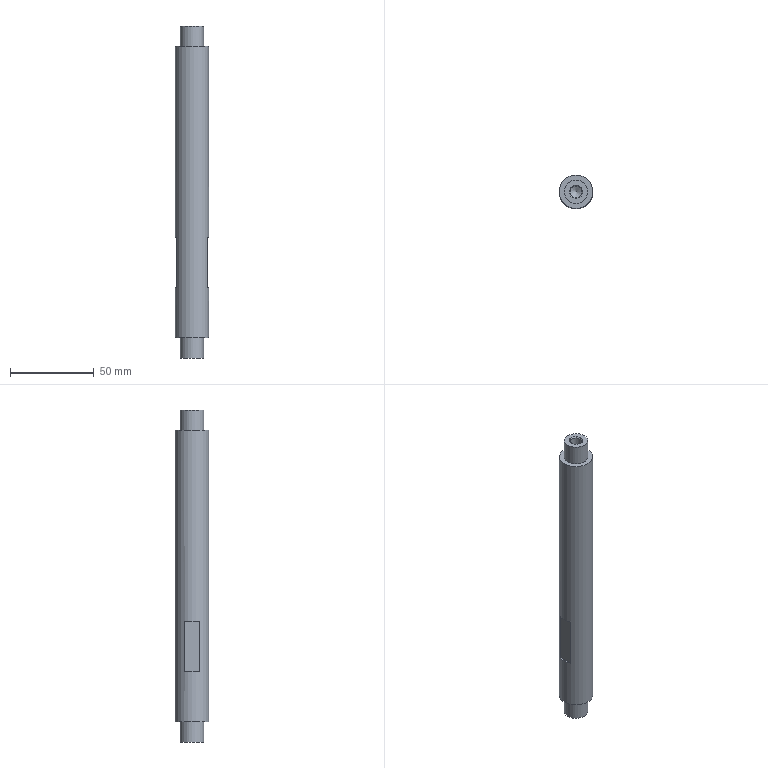Part | STEP file | YBQDJ-YL-9 | 1 solid | 16 faces | box 20 x 20 x 198 mm | volume 57396 mm3 | plane 10 | cylinder 4 | cone 2 | commonest cylinder face diameters 14 x2 6.8 x1 20 x1
STEP:
#1=CARTESIAN_POINT('',(0.,0.,0.));
#2=DIRECTION('',(0.,0.,1.));
#3=DIRECTION('',(1.,0.,0.));
#4=AXIS2_PLACEMENT_3D('',#1,#2,#3);
#5=CARTESIAN_POINT('',(231.5,-285.,50.));
#6=VERTEX_POINT('',#5);
#7=CARTESIAN_POINT('',(230.5,-280.641,50.));
#8=VERTEX_POINT('',#7);
#9=CARTESIAN_POINT('',(221.5,-285.,50.));
#10=DIRECTION('',(0.,0.,1.));
#11=DIRECTION('',(1.,0.,0.));
#12=AXIS2_PLACEMENT_3D('',#9,#10,#11);
#13=CIRCLE('',#12,10.);
#14=CARTESIAN_POINT('',(221.5,-285.,311.));
#15=DIRECTION('',(0.,0.,-1.));
#16=DIRECTION('',(1.,0.,0.));
#17=AXIS2_PLACEMENT_3D('',#14,#15,#16);
#18=CYLINDRICAL_SURFACE('',#17,10.);
#19=CARTESIAN_POINT('',(12.566,261.));
#20=DIRECTION('',(-1.,0.));
#21=VECTOR('',#20,1.);
#22=LINE('',#19,#21);
#23=(GEOMETRIC_REPRESENTATION_CONTEXT(2)PARAMETRIC_REPRESENTATION_CONTEXT()REPRESENTATION_CONTEXT('',''));
#24=DEFINITIONAL_REPRESENTATION('',(#22),#23);
#25=PCURVE('',#18,#24);
#26=CARTESIAN_POINT('',(230.5,-350.,50.));
#27=DIRECTION('',(0.,0.,1.));
#28=DIRECTION('',(1.,0.,0.));
#29=AXIS2_PLACEMENT_3D('',#26,#27,#28);
#30=PLANE('',#29);
#31=CARTESIAN_POINT('',(-9.,65.));
#32=DIRECTION('',(1.,0.));
#33=AXIS2_PLACEMENT_2D('',#31,#32);
#34=CIRCLE('',#33,10.);
#35=(GEOMETRIC_REPRESENTATION_CONTEXT(2)PARAMETRIC_REPRESENTATION_CONTEXT()REPRESENTATION_CONTEXT('',''));
#36=DEFINITIONAL_REPRESENTATION('',(#34),#35);
#37=PCURVE('',#30,#36);
#38=SURFACE_CURVE('',#13,(#25,#37),.PCURVE_S1.);
#39=EDGE_CURVE('',#6,#8,#38,.T.);
#40=ORIENTED_EDGE('',*,*,#39,.F.);
#41=CARTESIAN_POINT('',(231.5,-285.,20.));
#42=VERTEX_POINT('',#41);
#43=CARTESIAN_POINT('',(231.5,-285.,50.));
#44=CARTESIAN_POINT('',(231.5,-285.,20.));
#45=B_SPLINE_CURVE_WITH_KNOTS('',1,(#43,#44),.UNSPECIFIED.,.F.,.F.,(2,2),(261.,291.),.PIECEWISE_BEZIER_KNOTS.);
#46=CARTESIAN_POINT('',(6.283,0.));
#47=DIRECTION('',(0.,1.));
#48=VECTOR('',#47,1.);
#49=LINE('',#46,#48);
#50=(GEOMETRIC_REPRESENTATION_CONTEXT(2)PARAMETRIC_REPRESENTATION_CONTEXT()REPRESENTATION_CONTEXT('',''));
#51=DEFINITIONAL_REPRESENTATION('',(#49),#50);
#52=PCURVE('',#18,#51);
#53=CARTESIAN_POINT('',(0.,0.));
#54=DIRECTION('',(0.,1.));
#55=VECTOR('',#54,1.);
#56=LINE('',#53,#55);
#57=(GEOMETRIC_REPRESENTATION_CONTEXT(2)PARAMETRIC_REPRESENTATION_CONTEXT()REPRESENTATION_CONTEXT('',''));
#58=DEFINITIONAL_REPRESENTATION('',(#56),#57);
#59=PCURVE('',#18,#58);
#60=SEAM_CURVE('',#45,(#52,#59),.PCURVE_S1.);
#61=EDGE_CURVE('',#6,#42,#60,.T.);
#62=ORIENTED_EDGE('',*,*,#61,.T.);
#63=CARTESIAN_POINT('',(221.5,-285.,20.));
#64=DIRECTION('',(0.,0.,1.));
#65=DIRECTION('',(1.,0.,0.));
#66=AXIS2_PLACEMENT_3D('',#63,#64,#65);
#67=CIRCLE('',#66,10.);
#68=CARTESIAN_POINT('',(6.283,291.));
#69=DIRECTION('',(-1.,0.));
#70=VECTOR('',#69,1.);
#71=LINE('',#68,#70);
#72=(GEOMETRIC_REPRESENTATION_CONTEXT(2)PARAMETRIC_REPRESENTATION_CONTEXT()REPRESENTATION_CONTEXT('',''));
#73=DEFINITIONAL_REPRESENTATION('',(#71),#72);
#74=PCURVE('',#18,#73);
#75=CARTESIAN_POINT('',(131.5,-90.,20.));
#76=DIRECTION('',(0.,0.,1.));
#77=DIRECTION('',(0.,-1.,0.));
#78=AXIS2_PLACEMENT_3D('',#75,#76,#77);
#79=PLANE('',#78);
#80=CARTESIAN_POINT('',(195.,90.));
#81=DIRECTION('',(0.,1.));
#82=AXIS2_PLACEMENT_2D('',#80,#81);
#83=CIRCLE('',#82,10.);
#84=(GEOMETRIC_REPRESENTATION_CONTEXT(2)PARAMETRIC_REPRESENTATION_CONTEXT()REPRESENTATION_CONTEXT('',''));
#85=DEFINITIONAL_REPRESENTATION('',(#83),#84);
#86=PCURVE('',#79,#85);
#87=SURFACE_CURVE('',#67,(#74,#86),.PCURVE_S1.);
#88=EDGE_CURVE('',#42,#42,#87,.T.);
#89=ORIENTED_EDGE('',*,*,#88,.T.);
#90=ORIENTED_EDGE('',*,*,#61,.F.);
#91=CARTESIAN_POINT('',(230.5,-289.359,50.));
#92=VERTEX_POINT('',#91);
#93=CARTESIAN_POINT('',(221.5,-285.,50.));
#94=DIRECTION('',(0.,0.,1.));
#95=DIRECTION('',(1.,0.,0.));
#96=AXIS2_PLACEMENT_3D('',#93,#94,#95);
#97=CIRCLE('',#96,10.);
#98=CARTESIAN_POINT('',(6.283,261.));
#99=DIRECTION('',(-1.,0.));
#100=VECTOR('',#99,1.);
#101=LINE('',#98,#100);
#102=(GEOMETRIC_REPRESENTATION_CONTEXT(2)PARAMETRIC_REPRESENTATION_CONTEXT()REPRESENTATION_CONTEXT('',''));
#103=DEFINITIONAL_REPRESENTATION('',(#101),#102);
#104=PCURVE('',#18,#103);
#105=CARTESIAN_POINT('',(-9.,65.));
#106=DIRECTION('',(1.,0.));
#107=AXIS2_PLACEMENT_2D('',#105,#106);
#108=CIRCLE('',#107,10.);
#109=(GEOMETRIC_REPRESENTATION_CONTEXT(2)PARAMETRIC_REPRESENTATION_CONTEXT()REPRESENTATION_CONTEXT('',''));
#110=DEFINITIONAL_REPRESENTATION('',(#108),#109);
#111=PCURVE('',#30,#110);
#112=SURFACE_CURVE('',#97,(#104,#111),.PCURVE_S1.);
#113=EDGE_CURVE('',#92,#6,#112,.T.);
#114=ORIENTED_EDGE('',*,*,#113,.F.);
#115=CARTESIAN_POINT('',(230.5,-289.359,80.));
#116=VERTEX_POINT('',#115);
#117=CARTESIAN_POINT('',(230.5,-289.359,311.));
#118=DIRECTION('',(0.,0.,-1.));
#119=VECTOR('',#118,1.);
#120=LINE('',#117,#119);
#121=CARTESIAN_POINT('',(0.451,0.));
#122=DIRECTION('',(0.,1.));
#123=VECTOR('',#122,1.);
#124=LINE('',#121,#123);
#125=(GEOMETRIC_REPRESENTATION_CONTEXT(2)PARAMETRIC_REPRESENTATION_CONTEXT()REPRESENTATION_CONTEXT('',''));
#126=DEFINITIONAL_REPRESENTATION('',(#124),#125);
#127=PCURVE('',#18,#126);
#128=CARTESIAN_POINT('',(230.5,-350.,80.));
#129=DIRECTION('',(1.,0.,0.));
#130=DIRECTION('',(0.,0.,-1.));
#131=AXIS2_PLACEMENT_3D('',#128,#129,#130);
#132=PLANE('',#131);
#133=CARTESIAN_POINT('',(-231.,60.641));
#134=DIRECTION('',(1.,0.));
#135=VECTOR('',#134,1.);
#136=LINE('',#133,#135);
#137=(GEOMETRIC_REPRESENTATION_CONTEXT(2)PARAMETRIC_REPRESENTATION_CONTEXT()REPRESENTATION_CONTEXT('',''));
#138=DEFINITIONAL_REPRESENTATION('',(#136),#137);
#139=PCURVE('',#132,#138);
#140=SURFACE_CURVE('',#120,(#127,#139),.PCURVE_S1.);
#141=EDGE_CURVE('',#116,#92,#140,.T.);
#142=ORIENTED_EDGE('',*,*,#141,.F.);
#143=CARTESIAN_POINT('',(231.5,-285.,80.));
#144=VERTEX_POINT('',#143);
#145=CARTESIAN_POINT('',(221.5,-285.,80.));
#146=DIRECTION('',(0.,0.,-1.));
#147=DIRECTION('',(-1.,0.,0.));
#148=AXIS2_PLACEMENT_3D('',#145,#146,#147);
#149=CIRCLE('',#148,10.);
#150=CARTESIAN_POINT('',(-3.142,231.));
#151=DIRECTION('',(1.,0.));
#152=VECTOR('',#151,1.);
#153=LINE('',#150,#152);
#154=(GEOMETRIC_REPRESENTATION_CONTEXT(2)PARAMETRIC_REPRESENTATION_CONTEXT()REPRESENTATION_CONTEXT('',''));
#155=DEFINITIONAL_REPRESENTATION('',(#153),#154);
#156=PCURVE('',#18,#155);
#157=CARTESIAN_POINT('',(259.,-350.,80.));
#158=DIRECTION('',(0.,0.,-1.));
#159=DIRECTION('',(-1.,0.,0.));
#160=AXIS2_PLACEMENT_3D('',#157,#158,#159);
#161=PLANE('',#160);
#162=CARTESIAN_POINT('',(37.5,65.));
#163=DIRECTION('',(1.,0.));
#164=AXIS2_PLACEMENT_2D('',#162,#163);
#165=CIRCLE('',#164,10.);
#166=(GEOMETRIC_REPRESENTATION_CONTEXT(2)PARAMETRIC_REPRESENTATION_CONTEXT()REPRESENTATION_CONTEXT('',''));
#167=DEFINITIONAL_REPRESENTATION('',(#165),#166);
#168=PCURVE('',#161,#167);
#169=SURFACE_CURVE('',#149,(#156,#168),.PCURVE_S1.);
#170=EDGE_CURVE('',#144,#116,#169,.T.);
#171=ORIENTED_EDGE('',*,*,#170,.F.);
#172=CARTESIAN_POINT('',(231.5,-285.,194.));
#173=VERTEX_POINT('',#172);
#174=CARTESIAN_POINT('',(231.5,-285.,194.));
#175=CARTESIAN_POINT('',(231.5,-285.,80.));
#176=B_SPLINE_CURVE_WITH_KNOTS('',1,(#174,#175),.UNSPECIFIED.,.F.,.F.,(2,2),(117.,231.),.PIECEWISE_BEZIER_KNOTS.);
#177=CARTESIAN_POINT('',(0.,0.));
#178=DIRECTION('',(0.,1.));
#179=VECTOR('',#178,1.);
#180=LINE('',#177,#179);
#181=(GEOMETRIC_REPRESENTATION_CONTEXT(2)PARAMETRIC_REPRESENTATION_CONTEXT()REPRESENTATION_CONTEXT('',''));
#182=DEFINITIONAL_REPRESENTATION('',(#180),#181);
#183=PCURVE('',#18,#182);
#184=CARTESIAN_POINT('',(6.283,0.));
#185=DIRECTION('',(0.,1.));
#186=VECTOR('',#185,1.);
#187=LINE('',#184,#186);
#188=(GEOMETRIC_REPRESENTATION_CONTEXT(2)PARAMETRIC_REPRESENTATION_CONTEXT()REPRESENTATION_CONTEXT('',''));
#189=DEFINITIONAL_REPRESENTATION('',(#187),#188);
#190=PCURVE('',#18,#189);
#191=SEAM_CURVE('',#176,(#183,#190),.PCURVE_S1.);
#192=EDGE_CURVE('',#173,#144,#191,.T.);
#193=ORIENTED_EDGE('',*,*,#192,.F.);
#194=CARTESIAN_POINT('',(211.5,-285.,194.));
#195=VERTEX_POINT('',#194);
#196=CARTESIAN_POINT('',(221.5,-285.,194.));
#197=DIRECTION('',(0.,0.,1.));
#198=DIRECTION('',(-1.,0.,0.));
#199=AXIS2_PLACEMENT_3D('',#196,#197,#198);
#200=CIRCLE('',#199,10.);
#201=CARTESIAN_POINT('',(3.142,117.));
#202=DIRECTION('',(-1.,0.));
#203=VECTOR('',#202,1.);
#204=LINE('',#201,#203);
#205=(GEOMETRIC_REPRESENTATION_CONTEXT(2)PARAMETRIC_REPRESENTATION_CONTEXT()REPRESENTATION_CONTEXT('',''));
#206=DEFINITIONAL_REPRESENTATION('',(#204),#205);
#207=PCURVE('',#18,#206);
#208=CARTESIAN_POINT('',(365.5,-285.,194.));
#209=DIRECTION('',(0.,0.,-1.));
#210=DIRECTION('',(-1.,0.,0.));
#211=AXIS2_PLACEMENT_3D('',#208,#209,#210);
#212=PLANE('',#211);
#213=CARTESIAN_POINT('',(154.,0.));
#214=CARTESIAN_POINT('',(154.,-17.321));
#215=CARTESIAN_POINT('',(139.,-8.66));
#216=CARTESIAN_POINT('',(124.,0.));
#217=CARTESIAN_POINT('',(139.,8.66));
#218=CARTESIAN_POINT('',(154.,17.321));
#219=CARTESIAN_POINT('',(154.,0.));
#220=(BOUNDED_CURVE()B_SPLINE_CURVE(2,(#213,#214,#215,#216,#217,#218,#219),.UNSPECIFIED.,.T.,.F.)B_SPLINE_CURVE_WITH_KNOTS((1,2,2,2,2,1),(-2.094,0.,2.094,4.189,6.283,8.378),.UNSPECIFIED.)CURVE()GEOMETRIC_REPRESENTATION_ITEM()RATIONAL_B_SPLINE_CURVE((1.,0.5,1.,0.5,1.,0.5,1.))REPRESENTATION_ITEM(''));
#221=(GEOMETRIC_REPRESENTATION_CONTEXT(2)PARAMETRIC_REPRESENTATION_CONTEXT()REPRESENTATION_CONTEXT('',''));
#222=DEFINITIONAL_REPRESENTATION('',(#220),#221);
#223=PCURVE('',#212,#222);
#224=SURFACE_CURVE('',#200,(#207,#223),.PCURVE_S1.);
#225=EDGE_CURVE('',#195,#173,#224,.T.);
#226=ORIENTED_EDGE('',*,*,#225,.F.);
#227=CARTESIAN_POINT('',(221.5,-285.,194.));
#228=DIRECTION('',(0.,0.,1.));
#229=DIRECTION('',(-1.,0.,0.));
#230=AXIS2_PLACEMENT_3D('',#227,#228,#229);
#231=CIRCLE('',#230,10.);
#232=CARTESIAN_POINT('',(9.425,117.));
#233=DIRECTION('',(-1.,0.));
#234=VECTOR('',#233,1.);
#235=LINE('',#232,#234);
#236=(GEOMETRIC_REPRESENTATION_CONTEXT(2)PARAMETRIC_REPRESENTATION_CONTEXT()REPRESENTATION_CONTEXT('',''));
#237=DEFINITIONAL_REPRESENTATION('',(#235),#236);
#238=PCURVE('',#18,#237);
#239=CARTESIAN_POINT('',(154.,0.));
#240=CARTESIAN_POINT('',(154.,-17.321));
#241=CARTESIAN_POINT('',(139.,-8.66));
#242=CARTESIAN_POINT('',(124.,0.));
#243=CARTESIAN_POINT('',(139.,8.66));
#244=CARTESIAN_POINT('',(154.,17.321));
#245=CARTESIAN_POINT('',(154.,0.));
#246=(BOUNDED_CURVE()B_SPLINE_CURVE(2,(#239,#240,#241,#242,#243,#244,#245),.UNSPECIFIED.,.T.,.F.)B_SPLINE_CURVE_WITH_KNOTS((1,2,2,2,2,1),(-2.094,0.,2.094,4.189,6.283,8.378),.UNSPECIFIED.)CURVE()GEOMETRIC_REPRESENTATION_ITEM()RATIONAL_B_SPLINE_CURVE((1.,0.5,1.,0.5,1.,0.5,1.))REPRESENTATION_ITEM(''));
#247=(GEOMETRIC_REPRESENTATION_CONTEXT(2)PARAMETRIC_REPRESENTATION_CONTEXT()REPRESENTATION_CONTEXT('',''));
#248=DEFINITIONAL_REPRESENTATION('',(#246),#247);
#249=PCURVE('',#212,#248);
#250=SURFACE_CURVE('',#231,(#238,#249),.PCURVE_S1.);
#251=EDGE_CURVE('',#173,#195,#250,.T.);
#252=ORIENTED_EDGE('',*,*,#251,.F.);
#253=ORIENTED_EDGE('',*,*,#192,.T.);
#254=CARTESIAN_POINT('',(230.5,-280.641,80.));
#255=VERTEX_POINT('',#254);
#256=CARTESIAN_POINT('',(221.5,-285.,80.));
#257=DIRECTION('',(0.,0.,-1.));
#258=DIRECTION('',(-1.,0.,0.));
#259=AXIS2_PLACEMENT_3D('',#256,#257,#258);
#260=CIRCLE('',#259,10.);
#261=CARTESIAN_POINT('',(3.142,231.));
#262=DIRECTION('',(1.,0.));
#263=VECTOR('',#262,1.);
#264=LINE('',#261,#263);
#265=(GEOMETRIC_REPRESENTATION_CONTEXT(2)PARAMETRIC_REPRESENTATION_CONTEXT()REPRESENTATION_CONTEXT('',''));
#266=DEFINITIONAL_REPRESENTATION('',(#264),#265);
#267=PCURVE('',#18,#266);
#268=CARTESIAN_POINT('',(37.5,65.));
#269=DIRECTION('',(1.,0.));
#270=AXIS2_PLACEMENT_2D('',#268,#269);
#271=CIRCLE('',#270,10.);
#272=(GEOMETRIC_REPRESENTATION_CONTEXT(2)PARAMETRIC_REPRESENTATION_CONTEXT()REPRESENTATION_CONTEXT('',''));
#273=DEFINITIONAL_REPRESENTATION('',(#271),#272);
#274=PCURVE('',#161,#273);
#275=SURFACE_CURVE('',#260,(#267,#274),.PCURVE_S1.);
#276=EDGE_CURVE('',#255,#144,#275,.T.);
#277=ORIENTED_EDGE('',*,*,#276,.F.);
#278=CARTESIAN_POINT('',(230.5,-280.641,311.));
#279=DIRECTION('',(0.,0.,1.));
#280=VECTOR('',#279,1.);
#281=LINE('',#278,#280);
#282=CARTESIAN_POINT('',(5.832,0.));
#283=DIRECTION('',(0.,-1.));
#284=VECTOR('',#283,1.);
#285=LINE('',#282,#284);
#286=(GEOMETRIC_REPRESENTATION_CONTEXT(2)PARAMETRIC_REPRESENTATION_CONTEXT()REPRESENTATION_CONTEXT('',''));
#287=DEFINITIONAL_REPRESENTATION('',(#285),#286);
#288=PCURVE('',#18,#287);
#289=CARTESIAN_POINT('',(-231.,69.359));
#290=DIRECTION('',(-1.,0.));
#291=VECTOR('',#290,1.);
#292=LINE('',#289,#291);
#293=(GEOMETRIC_REPRESENTATION_CONTEXT(2)PARAMETRIC_REPRESENTATION_CONTEXT()REPRESENTATION_CONTEXT('',''));
#294=DEFINITIONAL_REPRESENTATION('',(#292),#293);
#295=PCURVE('',#132,#294);
#296=SURFACE_CURVE('',#281,(#288,#295),.PCURVE_S1.);
#297=EDGE_CURVE('',#8,#255,#296,.T.);
#298=ORIENTED_EDGE('',*,*,#297,.F.);
#299=EDGE_LOOP('',(#40,#62,#89,#90,#114,#142,#171,#193,#226,#252,#253,#277,#298));
#300=FACE_BOUND('',#299,.T.);
#301=CARTESIAN_POINT('',(212.5,-280.641,50.));
#302=VERTEX_POINT('',#301);
#303=CARTESIAN_POINT('',(212.5,-289.359,50.));
#304=VERTEX_POINT('',#303);
#305=CARTESIAN_POINT('',(221.5,-285.,50.));
#306=DIRECTION('',(0.,0.,1.));
#307=DIRECTION('',(1.,0.,0.));
#308=AXIS2_PLACEMENT_3D('',#305,#306,#307);
#309=CIRCLE('',#308,10.);
#310=CARTESIAN_POINT('',(6.283,261.));
#311=DIRECTION('',(-1.,0.));
#312=VECTOR('',#311,1.);
#313=LINE('',#310,#312);
#314=(GEOMETRIC_REPRESENTATION_CONTEXT(2)PARAMETRIC_REPRESENTATION_CONTEXT()REPRESENTATION_CONTEXT('',''));
#315=DEFINITIONAL_REPRESENTATION('',(#313),#314);
#316=PCURVE('',#18,#315);
#317=CARTESIAN_POINT('',(184.,-350.,50.));
#318=DIRECTION('',(0.,0.,1.));
#319=DIRECTION('',(1.,0.,0.));
#320=AXIS2_PLACEMENT_3D('',#317,#318,#319);
#321=PLANE('',#320);
#322=CARTESIAN_POINT('',(37.5,65.));
#323=DIRECTION('',(1.,0.));
#324=AXIS2_PLACEMENT_2D('',#322,#323);
#325=CIRCLE('',#324,10.);
#326=(GEOMETRIC_REPRESENTATION_CONTEXT(2)PARAMETRIC_REPRESENTATION_CONTEXT()REPRESENTATION_CONTEXT('',''));
#327=DEFINITIONAL_REPRESENTATION('',(#325),#326);
#328=PCURVE('',#321,#327);
#329=SURFACE_CURVE('',#309,(#316,#328),.PCURVE_S1.);
#330=EDGE_CURVE('',#302,#304,#329,.T.);
#331=ORIENTED_EDGE('',*,*,#330,.F.);
#332=CARTESIAN_POINT('',(212.5,-280.641,80.));
#333=VERTEX_POINT('',#332);
#334=CARTESIAN_POINT('',(212.5,-280.641,311.));
#335=DIRECTION('',(0.,0.,-1.));
#336=VECTOR('',#335,1.);
#337=LINE('',#334,#336);
#338=CARTESIAN_POINT('',(3.593,0.));
#339=DIRECTION('',(0.,1.));
#340=VECTOR('',#339,1.);
#341=LINE('',#338,#340);
#342=(GEOMETRIC_REPRESENTATION_CONTEXT(2)PARAMETRIC_REPRESENTATION_CONTEXT()REPRESENTATION_CONTEXT('',''));
#343=DEFINITIONAL_REPRESENTATION('',(#341),#342);
#344=PCURVE('',#18,#343);
#345=CARTESIAN_POINT('',(212.5,-350.,50.));
#346=DIRECTION('',(-1.,0.,0.));
#347=DIRECTION('',(0.,0.,1.));
#348=AXIS2_PLACEMENT_3D('',#345,#346,#347);
#349=PLANE('',#348);
#350=CARTESIAN_POINT('',(261.,69.359));
#351=DIRECTION('',(-1.,0.));
#352=VECTOR('',#351,1.);
#353=LINE('',#350,#352);
#354=(GEOMETRIC_REPRESENTATION_CONTEXT(2)PARAMETRIC_REPRESENTATION_CONTEXT()REPRESENTATION_CONTEXT('',''));
#355=DEFINITIONAL_REPRESENTATION('',(#353),#354);
#356=PCURVE('',#349,#355);
#357=SURFACE_CURVE('',#337,(#344,#356),.PCURVE_S1.);
#358=EDGE_CURVE('',#333,#302,#357,.T.);
#359=ORIENTED_EDGE('',*,*,#358,.F.);
#360=CARTESIAN_POINT('',(212.5,-289.359,80.));
#361=VERTEX_POINT('',#360);
#362=CARTESIAN_POINT('',(221.5,-285.,80.));
#363=DIRECTION('',(0.,0.,-1.));
#364=DIRECTION('',(-1.,0.,0.));
#365=AXIS2_PLACEMENT_3D('',#362,#363,#364);
#366=CIRCLE('',#365,10.);
#367=CARTESIAN_POINT('',(-3.142,231.));
#368=DIRECTION('',(1.,0.));
#369=VECTOR('',#368,1.);
#370=LINE('',#367,#369);
#371=(GEOMETRIC_REPRESENTATION_CONTEXT(2)PARAMETRIC_REPRESENTATION_CONTEXT()REPRESENTATION_CONTEXT('',''));
#372=DEFINITIONAL_REPRESENTATION('',(#370),#371);
#373=PCURVE('',#18,#372);
#374=CARTESIAN_POINT('',(212.5,-350.,80.));
#375=DIRECTION('',(0.,0.,-1.));
#376=DIRECTION('',(-1.,0.,0.));
#377=AXIS2_PLACEMENT_3D('',#374,#375,#376);
#378=PLANE('',#377);
#379=CARTESIAN_POINT('',(-9.,65.));
#380=DIRECTION('',(1.,0.));
#381=AXIS2_PLACEMENT_2D('',#379,#380);
#382=CIRCLE('',#381,10.);
#383=(GEOMETRIC_REPRESENTATION_CONTEXT(2)PARAMETRIC_REPRESENTATION_CONTEXT()REPRESENTATION_CONTEXT('',''));
#384=DEFINITIONAL_REPRESENTATION('',(#382),#383);
#385=PCURVE('',#378,#384);
#386=SURFACE_CURVE('',#366,(#373,#385),.PCURVE_S1.);
#387=EDGE_CURVE('',#361,#333,#386,.T.);
#388=ORIENTED_EDGE('',*,*,#387,.F.);
#389=CARTESIAN_POINT('',(212.5,-289.359,311.));
#390=DIRECTION('',(0.,0.,1.));
#391=VECTOR('',#390,1.);
#392=LINE('',#389,#391);
#393=CARTESIAN_POINT('',(2.691,0.));
#394=DIRECTION('',(0.,-1.));
#395=VECTOR('',#394,1.);
#396=LINE('',#393,#395);
#397=(GEOMETRIC_REPRESENTATION_CONTEXT(2)PARAMETRIC_REPRESENTATION_CONTEXT()REPRESENTATION_CONTEXT('',''));
#398=DEFINITIONAL_REPRESENTATION('',(#396),#397);
#399=PCURVE('',#18,#398);
#400=CARTESIAN_POINT('',(261.,60.641));
#401=DIRECTION('',(1.,0.));
#402=VECTOR('',#401,1.);
#403=LINE('',#400,#402);
#404=(GEOMETRIC_REPRESENTATION_CONTEXT(2)PARAMETRIC_REPRESENTATION_CONTEXT()REPRESENTATION_CONTEXT('',''));
#405=DEFINITIONAL_REPRESENTATION('',(#403),#404);
#406=PCURVE('',#349,#405);
#407=SURFACE_CURVE('',#392,(#399,#406),.PCURVE_S1.);
#408=EDGE_CURVE('',#304,#361,#407,.T.);
#409=ORIENTED_EDGE('',*,*,#408,.F.);
#410=EDGE_LOOP('',(#331,#359,#388,#409));
#411=FACE_BOUND('',#410,.T.);
#412=ADVANCED_FACE('',(#300,#411),#18,.T.);
#413=CARTESIAN_POINT('',(228.5,-285.,194.));
#414=VERTEX_POINT('',#413);
#415=CARTESIAN_POINT('',(221.5,-285.,194.));
#416=DIRECTION('',(0.,0.,1.));
#417=DIRECTION('',(1.,0.,0.));
#418=AXIS2_PLACEMENT_3D('',#415,#416,#417);
#419=CIRCLE('',#418,7.);
#420=CARTESIAN_POINT('',(137.,0.));
#421=CARTESIAN_POINT('',(137.,12.124));
#422=CARTESIAN_POINT('',(147.5,6.062));
#423=CARTESIAN_POINT('',(158.,0.));
#424=CARTESIAN_POINT('',(147.5,-6.062));
#425=CARTESIAN_POINT('',(137.,-12.124));
#426=CARTESIAN_POINT('',(137.,0.));
#427=(BOUNDED_CURVE()B_SPLINE_CURVE(2,(#420,#421,#422,#423,#424,#425,#426),.UNSPECIFIED.,.T.,.F.)B_SPLINE_CURVE_WITH_KNOTS((1,2,2,2,2,1),(-2.094,0.,2.094,4.189,6.283,8.378),.UNSPECIFIED.)CURVE()GEOMETRIC_REPRESENTATION_ITEM()RATIONAL_B_SPLINE_CURVE((1.,0.5,1.,0.5,1.,0.5,1.))REPRESENTATION_ITEM(''));
#428=(GEOMETRIC_REPRESENTATION_CONTEXT(2)PARAMETRIC_REPRESENTATION_CONTEXT()REPRESENTATION_CONTEXT('',''));
#429=DEFINITIONAL_REPRESENTATION('',(#427),#428);
#430=PCURVE('',#212,#429);
#431=CARTESIAN_POINT('',(221.5,-285.,206.));
#432=DIRECTION('',(0.,0.,-1.));
#433=DIRECTION('',(-1.,0.,0.));
#434=AXIS2_PLACEMENT_3D('',#431,#432,#433);
#435=CYLINDRICAL_SURFACE('',#434,7.);
#436=CARTESIAN_POINT('',(9.425,12.));
#437=DIRECTION('',(-1.,0.));
#438=VECTOR('',#437,1.);
#439=LINE('',#436,#438);
#440=(GEOMETRIC_REPRESENTATION_CONTEXT(2)PARAMETRIC_REPRESENTATION_CONTEXT()REPRESENTATION_CONTEXT('',''));
#441=DEFINITIONAL_REPRESENTATION('',(#439),#440);
#442=PCURVE('',#435,#441);
#443=SURFACE_CURVE('',#419,(#430,#442),.PCURVE_S1.);
#444=EDGE_CURVE('',#414,#414,#443,.T.);
#445=ORIENTED_EDGE('',*,*,#444,.F.);
#446=EDGE_LOOP('',(#445));
#447=FACE_BOUND('',#446,.T.);
#448=ORIENTED_EDGE('',*,*,#225,.T.);
#449=ORIENTED_EDGE('',*,*,#251,.T.);
#450=EDGE_LOOP('',(#448,#449));
#451=FACE_BOUND('',#450,.T.);
#452=ADVANCED_FACE('',(#447,#451),#212,.F.);
#453=CARTESIAN_POINT('',(214.5,-285.,20.));
#454=VERTEX_POINT('',#453);
#455=CARTESIAN_POINT('',(221.5,-285.,20.));
#456=DIRECTION('',(0.,0.,-1.));
#457=DIRECTION('',(-1.,0.,0.));
#458=AXIS2_PLACEMENT_3D('',#455,#456,#457);
#459=CIRCLE('',#458,7.);
#460=CARTESIAN_POINT('',(195.,83.));
#461=CARTESIAN_POINT('',(182.876,83.));
#462=CARTESIAN_POINT('',(188.938,93.5));
#463=CARTESIAN_POINT('',(195.,104.));
#464=CARTESIAN_POINT('',(201.062,93.5));
#465=CARTESIAN_POINT('',(207.124,83.));
#466=CARTESIAN_POINT('',(195.,83.));
#467=(BOUNDED_CURVE()B_SPLINE_CURVE(2,(#460,#461,#462,#463,#464,#465,#466),.UNSPECIFIED.,.T.,.F.)B_SPLINE_CURVE_WITH_KNOTS((1,2,2,2,2,1),(-2.094,0.,2.094,4.189,6.283,8.378),.UNSPECIFIED.)CURVE()GEOMETRIC_REPRESENTATION_ITEM()RATIONAL_B_SPLINE_CURVE((1.,0.5,1.,0.5,1.,0.5,1.))REPRESENTATION_ITEM(''));
#468=(GEOMETRIC_REPRESENTATION_CONTEXT(2)PARAMETRIC_REPRESENTATION_CONTEXT()REPRESENTATION_CONTEXT('',''));
#469=DEFINITIONAL_REPRESENTATION('',(#467),#468);
#470=PCURVE('',#79,#469);
#471=CARTESIAN_POINT('',(221.5,-285.,-2.));
#472=DIRECTION('',(0.,0.,1.));
#473=DIRECTION('',(1.,0.,0.));
#474=AXIS2_PLACEMENT_3D('',#471,#472,#473);
#475=CYLINDRICAL_SURFACE('',#474,7.);
#476=CARTESIAN_POINT('',(9.425,22.));
#477=DIRECTION('',(-1.,0.));
#478=VECTOR('',#477,1.);
#479=LINE('',#476,#478);
#480=(GEOMETRIC_REPRESENTATION_CONTEXT(2)PARAMETRIC_REPRESENTATION_CONTEXT()REPRESENTATION_CONTEXT('',''));
#481=DEFINITIONAL_REPRESENTATION('',(#479),#480);
#482=PCURVE('',#475,#481);
#483=SURFACE_CURVE('',#459,(#470,#482),.PCURVE_S1.);
#484=EDGE_CURVE('',#454,#454,#483,.T.);
#485=ORIENTED_EDGE('',*,*,#484,.F.);
#486=EDGE_LOOP('',(#485));
#487=FACE_BOUND('',#486,.T.);
#488=ORIENTED_EDGE('',*,*,#88,.F.);
#489=EDGE_LOOP('',(#488));
#490=FACE_BOUND('',#489,.T.);
#491=ADVANCED_FACE('',(#487,#490),#79,.F.);
#492=CARTESIAN_POINT('',(228.5,-285.,206.));
#493=VERTEX_POINT('',#492);
#494=CARTESIAN_POINT('',(221.5,-285.,206.));
#495=DIRECTION('',(0.,0.,1.));
#496=DIRECTION('',(1.,0.,0.));
#497=AXIS2_PLACEMENT_3D('',#494,#495,#496);
#498=CIRCLE('',#497,7.);
#499=CARTESIAN_POINT('',(9.425,0.));
#500=DIRECTION('',(-1.,0.));
#501=VECTOR('',#500,1.);
#502=LINE('',#499,#501);
#503=(GEOMETRIC_REPRESENTATION_CONTEXT(2)PARAMETRIC_REPRESENTATION_CONTEXT()REPRESENTATION_CONTEXT('',''));
#504=DEFINITIONAL_REPRESENTATION('',(#502),#503);
#505=PCURVE('',#435,#504);
#506=CARTESIAN_POINT('',(221.5,-285.,206.));
#507=DIRECTION('',(0.,0.,1.));
#508=DIRECTION('',(1.,0.,0.));
#509=AXIS2_PLACEMENT_3D('',#506,#507,#508);
#510=PLANE('',#509);
#511=CARTESIAN_POINT('',(0.,0.));
#512=DIRECTION('',(1.,0.));
#513=AXIS2_PLACEMENT_2D('',#511,#512);
#514=CIRCLE('',#513,7.);
#515=(GEOMETRIC_REPRESENTATION_CONTEXT(2)PARAMETRIC_REPRESENTATION_CONTEXT()REPRESENTATION_CONTEXT('',''));
#516=DEFINITIONAL_REPRESENTATION('',(#514),#515);
#517=PCURVE('',#510,#516);
#518=SURFACE_CURVE('',#498,(#505,#517),.PCURVE_S1.);
#519=EDGE_CURVE('',#493,#493,#518,.T.);
#520=ORIENTED_EDGE('',*,*,#519,.F.);
#521=CARTESIAN_POINT('',(228.5,-285.,206.));
#522=CARTESIAN_POINT('',(228.5,-285.,194.));
#523=B_SPLINE_CURVE_WITH_KNOTS('',1,(#521,#522),.UNSPECIFIED.,.F.,.F.,(2,2),(0.,12.),.PIECEWISE_BEZIER_KNOTS.);
#524=CARTESIAN_POINT('',(9.425,0.));
#525=DIRECTION('',(0.,1.));
#526=VECTOR('',#525,1.);
#527=LINE('',#524,#526);
#528=(GEOMETRIC_REPRESENTATION_CONTEXT(2)PARAMETRIC_REPRESENTATION_CONTEXT()REPRESENTATION_CONTEXT('',''));
#529=DEFINITIONAL_REPRESENTATION('',(#527),#528);
#530=PCURVE('',#435,#529);
#531=CARTESIAN_POINT('',(3.142,0.));
#532=DIRECTION('',(0.,1.));
#533=VECTOR('',#532,1.);
#534=LINE('',#531,#533);
#535=(GEOMETRIC_REPRESENTATION_CONTEXT(2)PARAMETRIC_REPRESENTATION_CONTEXT()REPRESENTATION_CONTEXT('',''));
#536=DEFINITIONAL_REPRESENTATION('',(#534),#535);
#537=PCURVE('',#435,#536);
#538=SEAM_CURVE('',#523,(#530,#537),.PCURVE_S1.);
#539=EDGE_CURVE('',#493,#414,#538,.T.);
#540=ORIENTED_EDGE('',*,*,#539,.T.);
#541=ORIENTED_EDGE('',*,*,#444,.T.);
#542=ORIENTED_EDGE('',*,*,#539,.F.);
#543=EDGE_LOOP('',(#520,#540,#541,#542));
#544=FACE_BOUND('',#543,.T.);
#545=ADVANCED_FACE('',(#544),#435,.T.);
#546=CARTESIAN_POINT('',(225.5,-285.,206.));
#547=VERTEX_POINT('',#546);
#548=CARTESIAN_POINT('',(221.5,-285.,206.));
#549=DIRECTION('',(0.,0.,-1.));
#550=DIRECTION('',(1.,0.,0.));
#551=AXIS2_PLACEMENT_3D('',#548,#549,#550);
#552=CIRCLE('',#551,4.);
#553=CARTESIAN_POINT('',(4.,0.));
#554=CARTESIAN_POINT('',(4.,-6.928));
#555=CARTESIAN_POINT('',(-2.,-3.464));
#556=CARTESIAN_POINT('',(-8.,0.));
#557=CARTESIAN_POINT('',(-2.,3.464));
#558=CARTESIAN_POINT('',(4.,6.928));
#559=CARTESIAN_POINT('',(4.,0.));
#560=(BOUNDED_CURVE()B_SPLINE_CURVE(2,(#553,#554,#555,#556,#557,#558,#559),.UNSPECIFIED.,.T.,.F.)B_SPLINE_CURVE_WITH_KNOTS((1,2,2,2,2,1),(-2.094,0.,2.094,4.189,6.283,8.378),.UNSPECIFIED.)CURVE()GEOMETRIC_REPRESENTATION_ITEM()RATIONAL_B_SPLINE_CURVE((1.,0.5,1.,0.5,1.,0.5,1.))REPRESENTATION_ITEM(''));
#561=(GEOMETRIC_REPRESENTATION_CONTEXT(2)PARAMETRIC_REPRESENTATION_CONTEXT()REPRESENTATION_CONTEXT('',''));
#562=DEFINITIONAL_REPRESENTATION('',(#560),#561);
#563=PCURVE('',#510,#562);
#564=CARTESIAN_POINT('',(221.5,-285.,206.));
#565=DIRECTION('',(0.,0.,1.));
#566=DIRECTION('',(1.,0.,0.));
#567=AXIS2_PLACEMENT_3D('',#564,#565,#566);
#568=CONICAL_SURFACE('',#567,4.,0.7854);
#569=CARTESIAN_POINT('',(6.283,0.));
#570=DIRECTION('',(-1.,0.));
#571=VECTOR('',#570,1.);
#572=LINE('',#569,#571);
#573=(GEOMETRIC_REPRESENTATION_CONTEXT(2)PARAMETRIC_REPRESENTATION_CONTEXT()REPRESENTATION_CONTEXT('',''));
#574=DEFINITIONAL_REPRESENTATION('',(#572),#573);
#575=PCURVE('',#568,#574);
#576=SURFACE_CURVE('',#552,(#563,#575),.PCURVE_S1.);
#577=EDGE_CURVE('',#547,#547,#576,.T.);
#578=ORIENTED_EDGE('',*,*,#577,.T.);
#579=EDGE_LOOP('',(#578));
#580=FACE_BOUND('',#579,.T.);
#581=ORIENTED_EDGE('',*,*,#519,.T.);
#582=EDGE_LOOP('',(#581));
#583=FACE_BOUND('',#582,.T.);
#584=ADVANCED_FACE('',(#580,#583),#510,.T.);
#585=CARTESIAN_POINT('',(224.9,-285.,190.));
#586=VERTEX_POINT('',#585);
#587=CARTESIAN_POINT('',(218.1,-285.,190.));
#588=VERTEX_POINT('',#587);
#589=CARTESIAN_POINT('',(221.5,-285.,190.));
#590=DIRECTION('',(0.,0.,1.));
#591=DIRECTION('',(-1.,0.,0.));
#592=AXIS2_PLACEMENT_3D('',#589,#590,#591);
#593=CIRCLE('',#592,3.4);
#594=CARTESIAN_POINT('',(221.5,-285.,190.));
#595=DIRECTION('',(0.,0.,1.));
#596=DIRECTION('',(1.,0.,0.));
#597=AXIS2_PLACEMENT_3D('',#594,#595,#596);
#598=CONICAL_SURFACE('',#597,3.4,1.03);
#599=CARTESIAN_POINT('',(-3.142,0.));
#600=DIRECTION('',(1.,0.));
#601=VECTOR('',#600,1.);
#602=LINE('',#599,#601);
#603=(GEOMETRIC_REPRESENTATION_CONTEXT(2)PARAMETRIC_REPRESENTATION_CONTEXT()REPRESENTATION_CONTEXT('',''));
#604=DEFINITIONAL_REPRESENTATION('',(#602),#603);
#605=PCURVE('',#598,#604);
#606=CARTESIAN_POINT('',(221.5,-285.,206.));
#607=DIRECTION('',(0.,0.,-1.));
#608=DIRECTION('',(-1.,0.,0.));
#609=AXIS2_PLACEMENT_3D('',#606,#607,#608);
#610=CYLINDRICAL_SURFACE('',#609,3.4);
#611=CARTESIAN_POINT('',(12.566,16.));
#612=DIRECTION('',(-1.,0.));
#613=VECTOR('',#612,1.);
#614=LINE('',#611,#613);
#615=(GEOMETRIC_REPRESENTATION_CONTEXT(2)PARAMETRIC_REPRESENTATION_CONTEXT()REPRESENTATION_CONTEXT('',''));
#616=DEFINITIONAL_REPRESENTATION('',(#614),#615);
#617=PCURVE('',#610,#616);
#618=SURFACE_CURVE('',#593,(#605,#617),.PCURVE_S1.);
#619=EDGE_CURVE('',#586,#588,#618,.T.);
#620=ORIENTED_EDGE('',*,*,#619,.F.);
#621=CARTESIAN_POINT('',(221.5,-285.,187.957));
#622=VERTEX_POINT('',#621);
#623=CARTESIAN_POINT('',(221.5,-285.,187.957));
#624=CARTESIAN_POINT('',(224.9,-285.,190.));
#625=B_SPLINE_CURVE_WITH_KNOTS('',1,(#623,#624),.UNSPECIFIED.,.F.,.F.,(2,2),(-3.967,0.),.PIECEWISE_BEZIER_KNOTS.);
#626=CARTESIAN_POINT('',(0.,0.));
#627=DIRECTION('',(0.,1.));
#628=VECTOR('',#627,1.);
#629=LINE('',#626,#628);
#630=(GEOMETRIC_REPRESENTATION_CONTEXT(2)PARAMETRIC_REPRESENTATION_CONTEXT()REPRESENTATION_CONTEXT('',''));
#631=DEFINITIONAL_REPRESENTATION('',(#629),#630);
#632=PCURVE('',#598,#631);
#633=CARTESIAN_POINT('',(6.283,0.));
#634=DIRECTION('',(0.,1.));
#635=VECTOR('',#634,1.);
#636=LINE('',#633,#635);
#637=(GEOMETRIC_REPRESENTATION_CONTEXT(2)PARAMETRIC_REPRESENTATION_CONTEXT()REPRESENTATION_CONTEXT('',''));
#638=DEFINITIONAL_REPRESENTATION('',(#636),#637);
#639=PCURVE('',#598,#638);
#640=SEAM_CURVE('',#625,(#632,#639),.PCURVE_S1.);
#641=EDGE_CURVE('',#622,#586,#640,.T.);
#642=ORIENTED_EDGE('',*,*,#641,.F.);
#643=ORIENTED_EDGE('',*,*,#641,.T.);
#644=CARTESIAN_POINT('',(221.5,-285.,190.));
#645=DIRECTION('',(0.,0.,1.));
#646=DIRECTION('',(-1.,0.,0.));
#647=AXIS2_PLACEMENT_3D('',#644,#645,#646);
#648=CIRCLE('',#647,3.4);
#649=CARTESIAN_POINT('',(3.142,0.));
#650=DIRECTION('',(1.,0.));
#651=VECTOR('',#650,1.);
#652=LINE('',#649,#651);
#653=(GEOMETRIC_REPRESENTATION_CONTEXT(2)PARAMETRIC_REPRESENTATION_CONTEXT()REPRESENTATION_CONTEXT('',''));
#654=DEFINITIONAL_REPRESENTATION('',(#652),#653);
#655=PCURVE('',#598,#654);
#656=CARTESIAN_POINT('',(6.283,16.));
#657=DIRECTION('',(-1.,0.));
#658=VECTOR('',#657,1.);
#659=LINE('',#656,#658);
#660=(GEOMETRIC_REPRESENTATION_CONTEXT(2)PARAMETRIC_REPRESENTATION_CONTEXT()REPRESENTATION_CONTEXT('',''));
#661=DEFINITIONAL_REPRESENTATION('',(#659),#660);
#662=PCURVE('',#610,#661);
#663=SURFACE_CURVE('',#648,(#655,#662),.PCURVE_S1.);
#664=EDGE_CURVE('',#588,#586,#663,.T.);
#665=ORIENTED_EDGE('',*,*,#664,.F.);
#666=EDGE_LOOP('',(#620,#642,#643,#665));
#667=FACE_BOUND('',#666,.F.);
#668=ADVANCED_FACE('',(#667),#598,.F.);
#669=CARTESIAN_POINT('',(224.9,-285.,205.4));
#670=VERTEX_POINT('',#669);
#671=CARTESIAN_POINT('',(221.5,-285.,205.4));
#672=DIRECTION('',(0.,0.,1.));
#673=DIRECTION('',(1.,0.,0.));
#674=AXIS2_PLACEMENT_3D('',#671,#672,#673);
#675=CIRCLE('',#674,3.4);
#676=CARTESIAN_POINT('',(9.425,0.6));
#677=DIRECTION('',(-1.,0.));
#678=VECTOR('',#677,1.);
#679=LINE('',#676,#678);
#680=(GEOMETRIC_REPRESENTATION_CONTEXT(2)PARAMETRIC_REPRESENTATION_CONTEXT()REPRESENTATION_CONTEXT('',''));
#681=DEFINITIONAL_REPRESENTATION('',(#679),#680);
#682=PCURVE('',#610,#681);
#683=CARTESIAN_POINT('',(0.,-0.6));
#684=DIRECTION('',(1.,0.));
#685=VECTOR('',#684,1.);
#686=LINE('',#683,#685);
#687=(GEOMETRIC_REPRESENTATION_CONTEXT(2)PARAMETRIC_REPRESENTATION_CONTEXT()REPRESENTATION_CONTEXT('',''));
#688=DEFINITIONAL_REPRESENTATION('',(#686),#687);
#689=PCURVE('',#568,#688);
#690=SURFACE_CURVE('',#675,(#682,#689),.PCURVE_S1.);
#691=EDGE_CURVE('',#670,#670,#690,.T.);
#692=ORIENTED_EDGE('',*,*,#691,.F.);
#693=CARTESIAN_POINT('',(224.9,-285.,205.4));
#694=CARTESIAN_POINT('',(224.9,-285.,190.));
#695=B_SPLINE_CURVE_WITH_KNOTS('',1,(#693,#694),.UNSPECIFIED.,.F.,.F.,(2,2),(0.6,16.),.PIECEWISE_BEZIER_KNOTS.);
#696=CARTESIAN_POINT('',(9.425,0.));
#697=DIRECTION('',(0.,1.));
#698=VECTOR('',#697,1.);
#699=LINE('',#696,#698);
#700=(GEOMETRIC_REPRESENTATION_CONTEXT(2)PARAMETRIC_REPRESENTATION_CONTEXT()REPRESENTATION_CONTEXT('',''));
#701=DEFINITIONAL_REPRESENTATION('',(#699),#700);
#702=PCURVE('',#610,#701);
#703=CARTESIAN_POINT('',(3.142,0.));
#704=DIRECTION('',(0.,1.));
#705=VECTOR('',#704,1.);
#706=LINE('',#703,#705);
#707=(GEOMETRIC_REPRESENTATION_CONTEXT(2)PARAMETRIC_REPRESENTATION_CONTEXT()REPRESENTATION_CONTEXT('',''));
#708=DEFINITIONAL_REPRESENTATION('',(#706),#707);
#709=PCURVE('',#610,#708);
#710=SEAM_CURVE('',#695,(#702,#709),.PCURVE_S1.);
#711=EDGE_CURVE('',#670,#586,#710,.T.);
#712=ORIENTED_EDGE('',*,*,#711,.T.);
#713=ORIENTED_EDGE('',*,*,#619,.T.);
#714=ORIENTED_EDGE('',*,*,#664,.T.);
#715=ORIENTED_EDGE('',*,*,#711,.F.);
#716=EDGE_LOOP('',(#692,#712,#713,#714,#715));
#717=FACE_BOUND('',#716,.F.);
#718=ADVANCED_FACE('',(#717),#610,.F.);
#719=ORIENTED_EDGE('',*,*,#691,.T.);
#720=CARTESIAN_POINT('',(224.9,-285.,205.4));
#721=CARTESIAN_POINT('',(225.5,-285.,206.));
#722=B_SPLINE_CURVE_WITH_KNOTS('',1,(#720,#721),.UNSPECIFIED.,.F.,.F.,(2,2),(-0.8485,0.),.PIECEWISE_BEZIER_KNOTS.);
#723=CARTESIAN_POINT('',(6.283,0.));
#724=DIRECTION('',(0.,1.));
#725=VECTOR('',#724,1.);
#726=LINE('',#723,#725);
#727=(GEOMETRIC_REPRESENTATION_CONTEXT(2)PARAMETRIC_REPRESENTATION_CONTEXT()REPRESENTATION_CONTEXT('',''));
#728=DEFINITIONAL_REPRESENTATION('',(#726),#727);
#729=PCURVE('',#568,#728);
#730=CARTESIAN_POINT('',(0.,0.));
#731=DIRECTION('',(0.,1.));
#732=VECTOR('',#731,1.);
#733=LINE('',#730,#732);
#734=(GEOMETRIC_REPRESENTATION_CONTEXT(2)PARAMETRIC_REPRESENTATION_CONTEXT()REPRESENTATION_CONTEXT('',''));
#735=DEFINITIONAL_REPRESENTATION('',(#733),#734);
#736=PCURVE('',#568,#735);
#737=SEAM_CURVE('',#722,(#729,#736),.PCURVE_S1.);
#738=EDGE_CURVE('',#670,#547,#737,.T.);
#739=ORIENTED_EDGE('',*,*,#738,.T.);
#740=ORIENTED_EDGE('',*,*,#577,.T.);
#741=ORIENTED_EDGE('',*,*,#738,.F.);
#742=EDGE_LOOP('',(#719,#739,#740,#741));
#743=FACE_BOUND('',#742,.F.);
#744=ADVANCED_FACE('',(#743),#568,.F.);
#745=CARTESIAN_POINT('',(214.5,-285.,8.));
#746=VERTEX_POINT('',#745);
#747=CARTESIAN_POINT('',(221.5,-285.,8.));
#748=DIRECTION('',(0.,0.,-1.));
#749=DIRECTION('',(-1.,0.,0.));
#750=AXIS2_PLACEMENT_3D('',#747,#748,#749);
#751=CIRCLE('',#750,7.);
#752=CARTESIAN_POINT('',(9.425,10.));
#753=DIRECTION('',(-1.,0.));
#754=VECTOR('',#753,1.);
#755=LINE('',#752,#754);
#756=(GEOMETRIC_REPRESENTATION_CONTEXT(2)PARAMETRIC_REPRESENTATION_CONTEXT()REPRESENTATION_CONTEXT('',''));
#757=DEFINITIONAL_REPRESENTATION('',(#755),#756);
#758=PCURVE('',#475,#757);
#759=CARTESIAN_POINT('',(221.5,-285.,8.));
#760=DIRECTION('',(0.,0.,-1.));
#761=DIRECTION('',(-1.,0.,0.));
#762=AXIS2_PLACEMENT_3D('',#759,#760,#761);
#763=PLANE('',#762);
#764=CARTESIAN_POINT('',(0.,0.));
#765=DIRECTION('',(1.,0.));
#766=AXIS2_PLACEMENT_2D('',#764,#765);
#767=CIRCLE('',#766,7.);
#768=(GEOMETRIC_REPRESENTATION_CONTEXT(2)PARAMETRIC_REPRESENTATION_CONTEXT()REPRESENTATION_CONTEXT('',''));
#769=DEFINITIONAL_REPRESENTATION('',(#767),#768);
#770=PCURVE('',#763,#769);
#771=SURFACE_CURVE('',#751,(#758,#770),.PCURVE_S1.);
#772=EDGE_CURVE('',#746,#746,#771,.T.);
#773=ORIENTED_EDGE('',*,*,#772,.F.);
#774=CARTESIAN_POINT('',(214.5,-285.,8.));
#775=CARTESIAN_POINT('',(214.5,-285.,20.));
#776=B_SPLINE_CURVE_WITH_KNOTS('',1,(#774,#775),.UNSPECIFIED.,.F.,.F.,(2,2),(10.,22.),.PIECEWISE_BEZIER_KNOTS.);
#777=CARTESIAN_POINT('',(9.425,0.));
#778=DIRECTION('',(0.,1.));
#779=VECTOR('',#778,1.);
#780=LINE('',#777,#779);
#781=(GEOMETRIC_REPRESENTATION_CONTEXT(2)PARAMETRIC_REPRESENTATION_CONTEXT()REPRESENTATION_CONTEXT('',''));
#782=DEFINITIONAL_REPRESENTATION('',(#780),#781);
#783=PCURVE('',#475,#782);
#784=CARTESIAN_POINT('',(3.142,0.));
#785=DIRECTION('',(0.,1.));
#786=VECTOR('',#785,1.);
#787=LINE('',#784,#786);
#788=(GEOMETRIC_REPRESENTATION_CONTEXT(2)PARAMETRIC_REPRESENTATION_CONTEXT()REPRESENTATION_CONTEXT('',''));
#789=DEFINITIONAL_REPRESENTATION('',(#787),#788);
#790=PCURVE('',#475,#789);
#791=SEAM_CURVE('',#776,(#783,#790),.PCURVE_S1.);
#792=EDGE_CURVE('',#746,#454,#791,.T.);
#793=ORIENTED_EDGE('',*,*,#792,.T.);
#794=ORIENTED_EDGE('',*,*,#484,.T.);
#795=ORIENTED_EDGE('',*,*,#792,.F.);
#796=EDGE_LOOP('',(#773,#793,#794,#795));
#797=FACE_BOUND('',#796,.T.);
#798=ADVANCED_FACE('',(#797),#475,.T.);
#799=ORIENTED_EDGE('',*,*,#772,.T.);
#800=EDGE_LOOP('',(#799));
#801=FACE_BOUND('',#800,.T.);
#802=ADVANCED_FACE('',(#801),#763,.T.);
#803=ORIENTED_EDGE('',*,*,#141,.T.);
#804=CARTESIAN_POINT('',(230.5,-350.,50.));
#805=DIRECTION('',(0.,-1.,0.));
#806=VECTOR('',#805,1.);
#807=LINE('',#804,#806);
#808=CARTESIAN_POINT('',(30.,0.));
#809=DIRECTION('',(0.,-1.));
#810=VECTOR('',#809,1.);
#811=LINE('',#808,#810);
#812=(GEOMETRIC_REPRESENTATION_CONTEXT(2)PARAMETRIC_REPRESENTATION_CONTEXT()REPRESENTATION_CONTEXT('',''));
#813=DEFINITIONAL_REPRESENTATION('',(#811),#812);
#814=PCURVE('',#132,#813);
#815=CARTESIAN_POINT('',(0.,0.));
#816=DIRECTION('',(0.,-1.));
#817=VECTOR('',#816,1.);
#818=LINE('',#815,#817);
#819=(GEOMETRIC_REPRESENTATION_CONTEXT(2)PARAMETRIC_REPRESENTATION_CONTEXT()REPRESENTATION_CONTEXT('',''));
#820=DEFINITIONAL_REPRESENTATION('',(#818),#819);
#821=PCURVE('',#30,#820);
#822=SURFACE_CURVE('',#807,(#814,#821),.PCURVE_S1.);
#823=EDGE_CURVE('',#8,#92,#822,.T.);
#824=ORIENTED_EDGE('',*,*,#823,.F.);
#825=ORIENTED_EDGE('',*,*,#297,.T.);
#826=CARTESIAN_POINT('',(230.5,-350.,80.));
#827=DIRECTION('',(0.,-1.,0.));
#828=VECTOR('',#827,1.);
#829=LINE('',#826,#828);
#830=CARTESIAN_POINT('',(0.,0.));
#831=DIRECTION('',(0.,-1.));
#832=VECTOR('',#831,1.);
#833=LINE('',#830,#832);
#834=(GEOMETRIC_REPRESENTATION_CONTEXT(2)PARAMETRIC_REPRESENTATION_CONTEXT()REPRESENTATION_CONTEXT('',''));
#835=DEFINITIONAL_REPRESENTATION('',(#833),#834);
#836=PCURVE('',#132,#835);
#837=CARTESIAN_POINT('',(28.5,0.));
#838=DIRECTION('',(0.,-1.));
#839=VECTOR('',#838,1.);
#840=LINE('',#837,#839);
#841=(GEOMETRIC_REPRESENTATION_CONTEXT(2)PARAMETRIC_REPRESENTATION_CONTEXT()REPRESENTATION_CONTEXT('',''));
#842=DEFINITIONAL_REPRESENTATION('',(#840),#841);
#843=PCURVE('',#161,#842);
#844=SURFACE_CURVE('',#829,(#836,#843),.PCURVE_S1.);
#845=EDGE_CURVE('',#255,#116,#844,.T.);
#846=ORIENTED_EDGE('',*,*,#845,.T.);
#847=EDGE_LOOP('',(#803,#824,#825,#846));
#848=FACE_BOUND('',#847,.T.);
#849=ADVANCED_FACE('',(#848),#132,.T.);
#850=ORIENTED_EDGE('',*,*,#113,.T.);
#851=ORIENTED_EDGE('',*,*,#39,.T.);
#852=ORIENTED_EDGE('',*,*,#823,.T.);
#853=EDGE_LOOP('',(#850,#851,#852));
#854=FACE_BOUND('',#853,.T.);
#855=ADVANCED_FACE('',(#854),#30,.T.);
#856=ORIENTED_EDGE('',*,*,#276,.T.);
#857=ORIENTED_EDGE('',*,*,#170,.T.);
#858=ORIENTED_EDGE('',*,*,#845,.F.);
#859=EDGE_LOOP('',(#856,#857,#858));
#860=FACE_BOUND('',#859,.T.);
#861=ADVANCED_FACE('',(#860),#161,.T.);
#862=ORIENTED_EDGE('',*,*,#330,.T.);
#863=CARTESIAN_POINT('',(212.5,-350.,50.));
#864=DIRECTION('',(0.,-1.,0.));
#865=VECTOR('',#864,1.);
#866=LINE('',#863,#865);
#867=CARTESIAN_POINT('',(28.5,0.));
#868=DIRECTION('',(0.,-1.));
#869=VECTOR('',#868,1.);
#870=LINE('',#867,#869);
#871=(GEOMETRIC_REPRESENTATION_CONTEXT(2)PARAMETRIC_REPRESENTATION_CONTEXT()REPRESENTATION_CONTEXT('',''));
#872=DEFINITIONAL_REPRESENTATION('',(#870),#871);
#873=PCURVE('',#321,#872);
#874=CARTESIAN_POINT('',(0.,0.));
#875=DIRECTION('',(0.,-1.));
#876=VECTOR('',#875,1.);
#877=LINE('',#874,#876);
#878=(GEOMETRIC_REPRESENTATION_CONTEXT(2)PARAMETRIC_REPRESENTATION_CONTEXT()REPRESENTATION_CONTEXT('',''));
#879=DEFINITIONAL_REPRESENTATION('',(#877),#878);
#880=PCURVE('',#349,#879);
#881=SURFACE_CURVE('',#866,(#873,#880),.PCURVE_S1.);
#882=EDGE_CURVE('',#302,#304,#881,.T.);
#883=ORIENTED_EDGE('',*,*,#882,.F.);
#884=EDGE_LOOP('',(#862,#883));
#885=FACE_BOUND('',#884,.T.);
#886=ADVANCED_FACE('',(#885),#321,.T.);
#887=ORIENTED_EDGE('',*,*,#358,.T.);
#888=ORIENTED_EDGE('',*,*,#882,.T.);
#889=ORIENTED_EDGE('',*,*,#408,.T.);
#890=CARTESIAN_POINT('',(212.5,-350.,80.));
#891=DIRECTION('',(0.,-1.,0.));
#892=VECTOR('',#891,1.);
#893=LINE('',#890,#892);
#894=CARTESIAN_POINT('',(30.,0.));
#895=DIRECTION('',(0.,-1.));
#896=VECTOR('',#895,1.);
#897=LINE('',#894,#896);
#898=(GEOMETRIC_REPRESENTATION_CONTEXT(2)PARAMETRIC_REPRESENTATION_CONTEXT()REPRESENTATION_CONTEXT('',''));
#899=DEFINITIONAL_REPRESENTATION('',(#897),#898);
#900=PCURVE('',#349,#899);
#901=CARTESIAN_POINT('',(0.,0.));
#902=DIRECTION('',(0.,-1.));
#903=VECTOR('',#902,1.);
#904=LINE('',#901,#903);
#905=(GEOMETRIC_REPRESENTATION_CONTEXT(2)PARAMETRIC_REPRESENTATION_CONTEXT()REPRESENTATION_CONTEXT('',''));
#906=DEFINITIONAL_REPRESENTATION('',(#904),#905);
#907=PCURVE('',#378,#906);
#908=SURFACE_CURVE('',#893,(#900,#907),.PCURVE_S1.);
#909=EDGE_CURVE('',#333,#361,#908,.T.);
#910=ORIENTED_EDGE('',*,*,#909,.F.);
#911=EDGE_LOOP('',(#887,#888,#889,#910));
#912=FACE_BOUND('',#911,.T.);
#913=ADVANCED_FACE('',(#912),#349,.T.);
#914=ORIENTED_EDGE('',*,*,#387,.T.);
#915=ORIENTED_EDGE('',*,*,#909,.T.);
#916=EDGE_LOOP('',(#914,#915));
#917=FACE_BOUND('',#916,.T.);
#918=ADVANCED_FACE('',(#917),#378,.T.);
#919=CLOSED_SHELL('',(#412,#452,#491,#545,#584,#668,#718,#744,#798,#802,#849,#855,#861,#886,#913,#918));
#920=MANIFOLD_SOLID_BREP('',#919);
#921=(LENGTH_UNIT()NAMED_UNIT(*)SI_UNIT(.MILLI.,.METRE.));
#922=UNCERTAINTY_MEASURE_WITH_UNIT(LENGTH_MEASURE(0.000005),#921,'','');
#923=(NAMED_UNIT(*)PLANE_ANGLE_UNIT()SI_UNIT($,.RADIAN.));
#924=(NAMED_UNIT(*)SI_UNIT($,.STERADIAN.)SOLID_ANGLE_UNIT());
#925=(GEOMETRIC_REPRESENTATION_CONTEXT(3)GLOBAL_UNCERTAINTY_ASSIGNED_CONTEXT((#922))GLOBAL_UNIT_ASSIGNED_CONTEXT((#921,#923,#924))REPRESENTATION_CONTEXT('',''));
#926=ADVANCED_BREP_SHAPE_REPRESENTATION('',(#4,#920),#925);